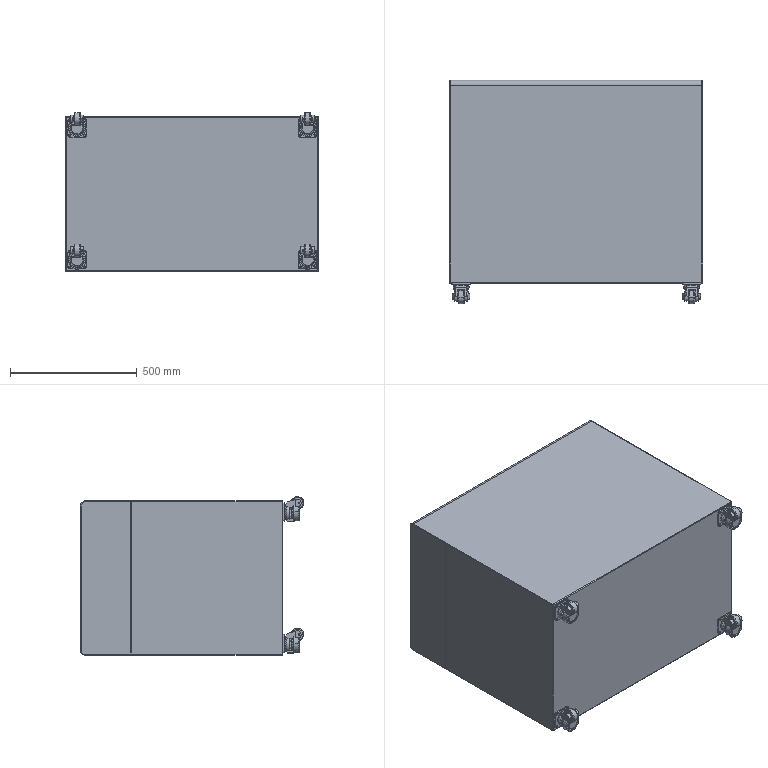Part | NX | features BREP 25 | 25 solids | 1203 faces | box 1000 x 882 x 627.5 mm | volume 488756342 mm3 | plane 519 | cylinder 344 | cone 272 | torus 64 | sphere 4 | commonest cylinder face diameters 7 x32 10 x32 35 x32 52 x32 6 x26 3 x24